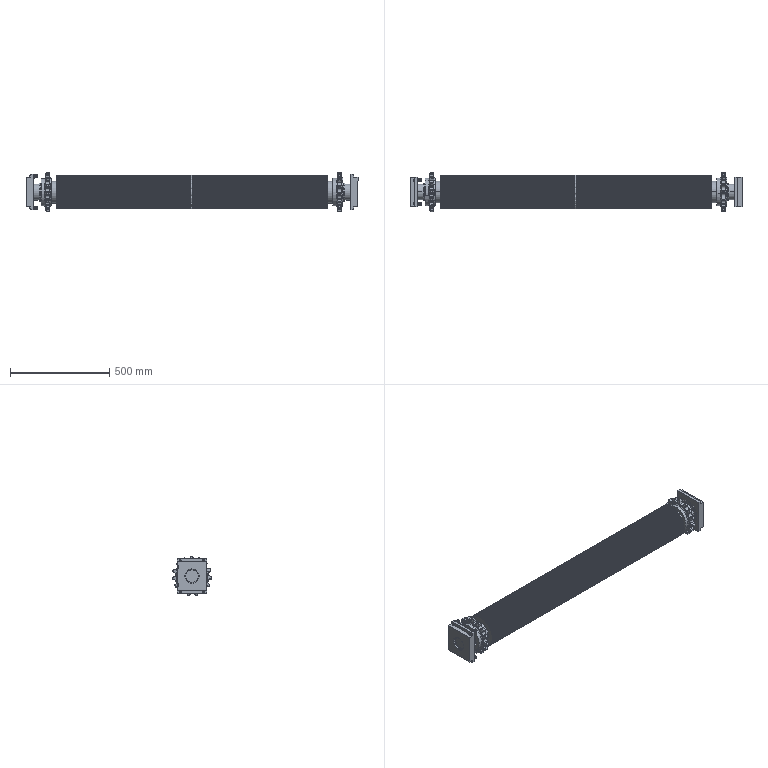Part | SolidWorks | 52 solids | 1725 faces | box 1672 x 198.631 x 197.926 mm | volume 35053418 mm3 | cylinder 1011 | plane 274 | cone 164 | sphere 144 | torus 132 | commonest cylinder face diameters 1 x288 2 x167 170 x120 89.75 x66 95.25 x66 32.838 x64